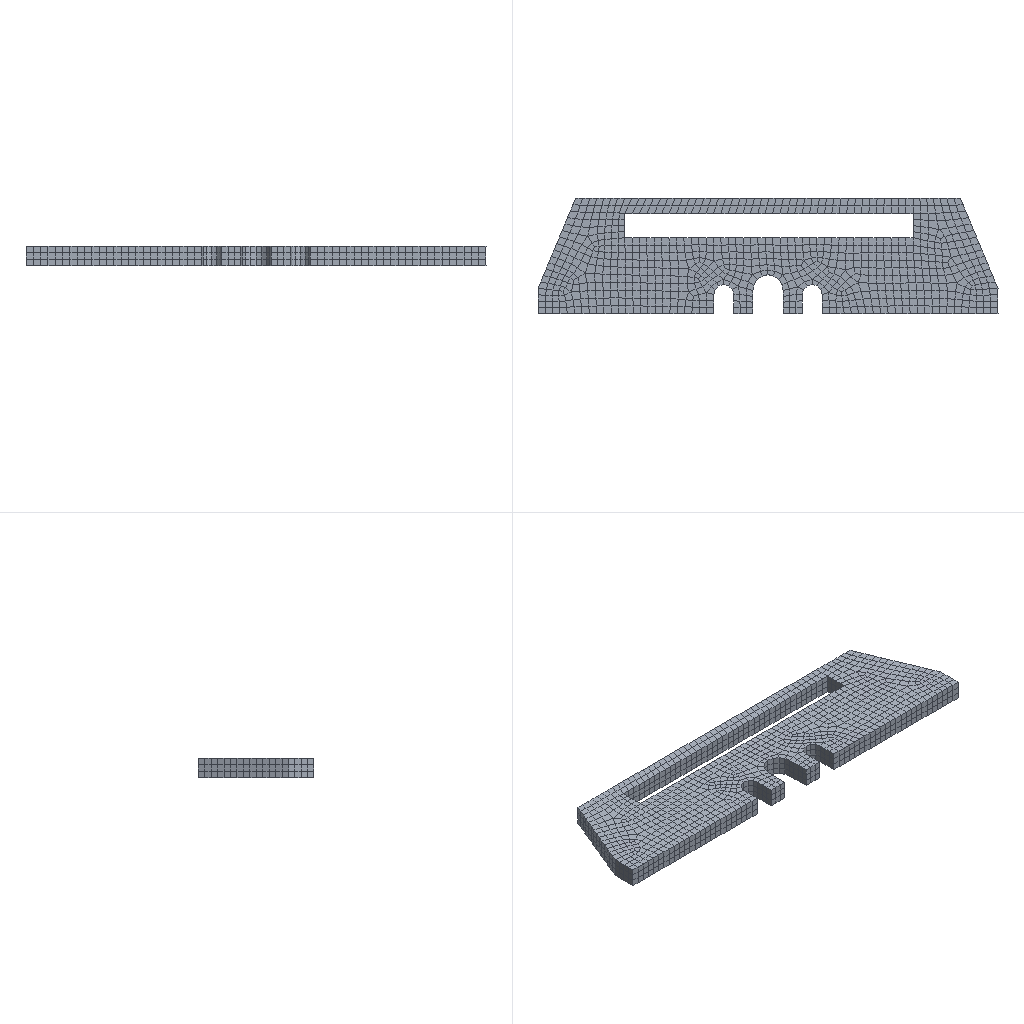Simulation study | ansys workbench
Ansys APDL input file, long lists of numbers shortened:
/batch
/config,noeldb,1     ! force off writing results to database
*get,_wallstrt,active,,time,wall
! ANSYS input file written by Workbench version 17.0 RELEASE
! File used for geometry attach:
/title,The wall thermal analysis--Static Structural (B5)
*DIM,_wb_ProjectScratch_dir,string,248
_wb_ProjectScratch_dir(1) = ''
*DIM,_wb_SolverFiles_dir,string,248
_wb_SolverFiles_dir(1) = ''
*DIM,_wb_userfiles_dir,string,248
_wb_userfiles_dir(1) = ''
/com,--- Data in consistent NMM units. See Solving Units in the help system for more information.
/units,MPA
/nopr
/wb,file,start              !  signify a WB generated input file
/prep7
! Turn off shape checking because checks already performed inside WB mesher.
! See help system for more information.
SHPP,OFF,,NOWARN
/nolist
etcon,set             ! allow ANSYS to choose best KEYOP's for 180x elements
/com,*********** Nodes for the whole assembly ***********
nblock,3
(1i9,3e20.9e3)
        1    1.298159564E+004    3.180623967E+003    0.000000000E+000
! (13514 more lines like these left out)
-1
/wb,elem,start            !  set before creation of elements
/com,*********** Elements for Body 1 "Wall" ***********
et,1,186
keyo,1,2,1          ! set full integration on SOLID186
eblock,19,solid,,2406
(19i9)
        1        1        1        1        0        0        0        0       20        0        1     2811     2810     2434     2641     3748     3747     3371     3578
! (4811 more lines like these left out)
-1
/wb,elem,end               !  done creating elements
/com,*********** Send User Defined Coordinate System(s) ***********
csys,0
toffst,273.15,  ! Temperature offset from absolute zero
/com,*********** Set Reference Temperature ***********
tref,22.
/wb,mat,start              !  starting to send materials
/com,*********** Send Materials ***********
MP,DENS,1,1.64e-09,	! tonne mm^-3
MP,ALPX,1,5e-06,	! C^-1
MP,C,1,960000000,	! mm^2 s^-2 C^-1
MP,KXX,1,52.78,	! tonne mm s^-3 C^-1
MP,EX,1,2230,	! tonne s^-2 mm^-1
MP,NUXY,1,0.1,
/wb,mat,end                !  done sending materials
!************************* Model Summary ********************
!Wall,	wall,	matid,	1
!************************* End Model Summary ********************
! get the diagonal of the bounding box. Needed later for other things
*get,_xmin,node,,mnloc,x
*get,_ymin,node,,mnloc,y
*get,_zmin,node,,mnloc,z
*get,_xmax,node,,mxloc,x
*get,_ymax,node,,mxloc,y
*get,_zmax,node,,mxloc,z
_ASMDIAG=(_xmax-_xmin)*(_xmax-_xmin)+(_ymax-_ymin)*(_ymax-_ymin)+(_zmax-_zmin)*(_zmax-_zmin)
_ASMDIAG=SQRT(_ASMDIAG)
/wb,contact,start          !  starting to send contact
/wb,contact,end            !  done creating contacts
/golist
/wb,load,start             !  starting to send loads
/com,******* Constant Zero Displacement X *******
CMBLOCK,_DISPZEROUX,NODE,      622
(8i10)
      1251      1252      1253      1254      1255      1256      1257      1258
! (77 more lines like these left out)
cmsel,s,_DISPZEROUX
d,all,ux,0
nsel,all
/com,******* Constant Zero Displacement Y *******
CMBLOCK,_DISPZEROUY,NODE,      622
(8i10)
      1251      1252      1253      1254      1255      1256      1257      1258
! (77 more lines like these left out)
cmsel,s,_DISPZEROUY
d,all,uy,0
nsel,all
/com,******* Constant Zero Displacement Z *******
CMBLOCK,_DISPZEROUZ,NODE,      622
(8i10)
      1251      1252      1253      1254      1255      1256      1257      1258
! (77 more lines like these left out)
cmsel,s,_DISPZEROUZ
d,all,uz,0
nsel,all
nsel,all
/com,*********** Define Pressure Using Surface Effect Elements ***********
et,2,154
eblock,10,,,802
(15i9)
     2407        2        2        2        0     1871     1873     1532     1118     3956     3949     7823     8476
! (801 more lines like these left out)
-1
esel,s,type,,2
esel,all
*DIM,_loadvari230,TABLE,2,2,1,Y,TIME
! Time Values
_loadvari230(0,1,1) = 0.
_loadvari230(0,2,1) = 1.
! Y values
_loadvari230(1,0,1) = 0.
_loadvari230(2,0,1) = 12000.
! Load values
_loadvari230(1,1,1) = 0.
_loadvari230(1,2,1) = 1.e-002
_loadvari230(2,1,1) = 0.
_loadvari230(2,2,1) = 2.5e-002
esel,all
/gst,on,on
fini
*get,_numnode,node,0,count
*get,_numelem,elem,0,count
*get, _MAXELEMNUM, elem, 0, NUM, MAX
*get, _MAXNODENUM, node, 0, NUM, MAX
*get, _MAXELEMTYPE, etyp, 0, NUM, MAX
*get, _MAXREALCONST, real, 0, NUM, MAX
/go
/wb,load,end               !  done creating loads
/com,--- Number of total nodes = %_numnode%
/com,--- Number of contact elements = 802
/com,--- Number of spring elements = 0
/com,--- Number of bearing elements = 0
/com,--- Number of solid elements = 2406
/com,--- Number of total elements = %_numelem%
*get,_wallbsol,active,,time,wall
/com,****************************************************************************
/com,*************************    SOLUTION       ********************************
/com,****************************************************************************
/solu
antype,0                   ! static analysis
eqsl,pcg,1e-8,,,,,,1
cntr,print,1               ! print out contact info and also make no initial contact an error
dmpopt,emat,no             ! Don't combine emat file for DANSYS
dmpopt,esav,no             ! Don't combine esav file for DANSYS
nldiag,cont,iter           ! print out contact info each equilibrium iteration
resc,,none                 ! Do not keep any restart files
/com,****************************************************
/com,******************* SOLVE FOR LS 1 ****************
esel,s,type,,2
nsle
sf,all,pres,%_loadvari230%
nsel,all
esel,all
esel,all
/nopr
/gopr
/com,*********** Create Imported Load "Imported Body Temperature" ***********
/nopr
bf,1,temp,-14.314
bf,2,temp,-14.318
bf,3,temp,-14.263
bf,4,temp,-14.267
! (13511 more lines like these left out)
/gopr
nsub,1,1,1
time,1.
outres,erase
outres,all,none
outres,nsol,all
outres,rsol,all
outres,strs,all
outres,epel,all
outres,eppl,all
outres,epth,all
stabilize,off                   ! Stabilization turned OFF by user
! *********** WB SOLVE COMMAND ***********
! check interactive state
*get,ANSINTER_,active,,int
*if,ANSINTER_,ne,0,then
/eof
*endif
solve
/com *************** Write FE CONNECTORS *********
CEWRITE,file,ce,,INTE
/com,****************************************************
/com,*************** FINISHED SOLVE FOR LS 1 *************
*set,_DS_PROGRESS          ! turn off progress updates to avoid virus scanning bug
*get,_wallasol,active,,time,wall
/nopr
*get,_numnode,node,0,count
*get,_numelem,elem,0,count
*get, _MAXELEMNUM, elem, 0, NUM, MAX
*get, _MAXNODENUM, node, 0, NUM, MAX,,,INTERNAL
*get, _MAXELEMTYPE, etyp, 0, NUM, MAX
*get, _MAXREALCONST, real, 0, NUM, MAX
/gopr
*get,_PCGITER,active,,solu,cgiter
/post1
xmlo,ENCODING,ISO-8859-1
xmlo,parm
/xml,parm,xml
fini
/gopr
*get,_walldone,active,,time,wall
_preptime=(_wallbsol-_wallstrt)*3600
_solvtime=(_wallasol-_wallbsol)*3600
_posttime=(_walldone-_wallasol)*3600
_totaltim=(_walldone-_wallstrt)*3600
/wb,file,end               ! done with WB generated input